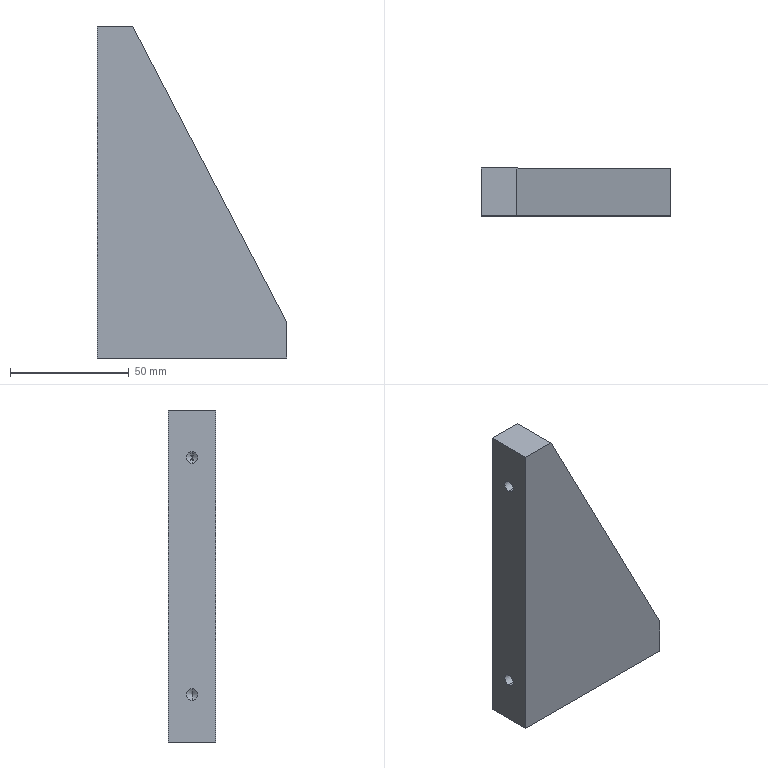Part | SolidWorks | features HoleWzd 2, Extrusion 1, ICE 1 | 1 solid | 23 faces | box 80 x 20 x 140 mm | volume 141533 mm3 | cylinder 8 | cone 8 | plane 7 | commonest cylinder face diameters 5 x8
STEP:
#1=CARTESIAN_POINT('',(75.,10.,-125.));
#2=VERTEX_POINT('',#1);
#3=CARTESIAN_POINT('',(70.,10.,-125.));
#4=VERTEX_POINT('',#3);
#5=CARTESIAN_POINT('',(72.5,10.,-125.));
#6=DIRECTION('',(0.,0.,-1.));
#7=DIRECTION('',(-1.,0.,0.));
#8=AXIS2_PLACEMENT_3D('',#5,#6,#7);
#9=CIRCLE('',#8,2.5);
#10=EDGE_CURVE('',#2,#4,#9,.T.);
#11=ORIENTED_EDGE('',*,*,#10,.F.);
#12=CARTESIAN_POINT('',(75.,10.,-140.));
#13=VERTEX_POINT('',#12);
#14=CARTESIAN_POINT('',(75.,10.,-140.));
#15=DIRECTION('',(0.,0.,-1.));
#16=VECTOR('',#15,1000.);
#17=LINE('',#14,#16);
#18=EDGE_CURVE('',#2,#13,#17,.T.);
#19=ORIENTED_EDGE('',*,*,#18,.T.);
#20=CARTESIAN_POINT('',(70.,10.,-140.));
#21=VERTEX_POINT('',#20);
#22=CARTESIAN_POINT('',(72.5,10.,-140.));
#23=DIRECTION('',(0.,0.,-1.));
#24=DIRECTION('',(-1.,0.,0.));
#25=AXIS2_PLACEMENT_3D('',#22,#23,#24);
#26=CIRCLE('',#25,2.5);
#27=EDGE_CURVE('',#13,#21,#26,.T.);
#28=ORIENTED_EDGE('',*,*,#27,.T.);
#29=CARTESIAN_POINT('',(70.,10.,-140.));
#30=DIRECTION('',(0.,0.,-1.));
#31=VECTOR('',#30,1000.);
#32=LINE('',#29,#31);
#33=EDGE_CURVE('',#4,#21,#32,.T.);
#34=ORIENTED_EDGE('',*,*,#33,.F.);
#35=EDGE_LOOP('',(#11,#19,#28,#34));
#36=FACE_OUTER_BOUND('',#35,.T.);
#37=CARTESIAN_POINT('',(72.5,10.,-140.));
#38=DIRECTION('',(0.,0.,-1.));
#39=DIRECTION('',(-1.,0.,0.));
#40=AXIS2_PLACEMENT_3D('',#37,#38,#39);
#41=CYLINDRICAL_SURFACE('',#40,2.5);
#42=ADVANCED_FACE('',(#36),#41,.F.);
#43=CARTESIAN_POINT('',(72.5,10.,-123.498));
#44=VERTEX_POINT('',#43);
#45=CARTESIAN_POINT('',(70.,10.,-125.));
#46=DIRECTION('',(-0.8572,0.,-0.515));
#47=VECTOR('',#46,1000.);
#48=LINE('',#45,#47);
#49=EDGE_CURVE('',#44,#4,#48,.T.);
#50=ORIENTED_EDGE('',*,*,#49,.F.);
#51=CARTESIAN_POINT('',(75.,10.,-125.));
#52=DIRECTION('',(0.8572,0.,-0.515));
#53=VECTOR('',#52,1000.);
#54=LINE('',#51,#53);
#55=EDGE_CURVE('',#44,#2,#54,.T.);
#56=ORIENTED_EDGE('',*,*,#55,.T.);
#57=ORIENTED_EDGE('',*,*,#10,.T.);
#58=EDGE_LOOP('',(#50,#56,#57));
#59=FACE_OUTER_BOUND('',#58,.T.);
#60=CARTESIAN_POINT('',(72.5,10.,-125.));
#61=DIRECTION('',(0.,0.,-1.));
#62=DIRECTION('',(-1.,0.,0.));
#63=AXIS2_PLACEMENT_3D('',#60,#61,#62);
#64=CONICAL_SURFACE('',#63,2.5,1.03);
#65=ADVANCED_FACE('',(#59),#64,.F.);
#66=CARTESIAN_POINT('',(10.,10.,-125.));
#67=VERTEX_POINT('',#66);
#68=CARTESIAN_POINT('',(5.,10.,-125.));
#69=VERTEX_POINT('',#68);
#70=CARTESIAN_POINT('',(7.5,10.,-125.));
#71=DIRECTION('',(0.,0.,-1.));
#72=DIRECTION('',(-1.,0.,0.));
#73=AXIS2_PLACEMENT_3D('',#70,#71,#72);
#74=CIRCLE('',#73,2.5);
#75=EDGE_CURVE('',#67,#69,#74,.T.);
#76=ORIENTED_EDGE('',*,*,#75,.F.);
#77=CARTESIAN_POINT('',(10.,10.,-140.));
#78=VERTEX_POINT('',#77);
#79=CARTESIAN_POINT('',(10.,10.,-140.));
#80=DIRECTION('',(0.,0.,-1.));
#81=VECTOR('',#80,1000.);
#82=LINE('',#79,#81);
#83=EDGE_CURVE('',#67,#78,#82,.T.);
#84=ORIENTED_EDGE('',*,*,#83,.T.);
#85=CARTESIAN_POINT('',(5.,10.,-140.));
#86=VERTEX_POINT('',#85);
#87=CARTESIAN_POINT('',(7.5,10.,-140.));
#88=DIRECTION('',(0.,0.,-1.));
#89=DIRECTION('',(-1.,0.,0.));
#90=AXIS2_PLACEMENT_3D('',#87,#88,#89);
#91=CIRCLE('',#90,2.5);
#92=EDGE_CURVE('',#78,#86,#91,.T.);
#93=ORIENTED_EDGE('',*,*,#92,.T.);
#94=CARTESIAN_POINT('',(5.,10.,-140.));
#95=DIRECTION('',(0.,0.,-1.));
#96=VECTOR('',#95,1000.);
#97=LINE('',#94,#96);
#98=EDGE_CURVE('',#69,#86,#97,.T.);
#99=ORIENTED_EDGE('',*,*,#98,.F.);
#100=EDGE_LOOP('',(#76,#84,#93,#99));
#101=FACE_OUTER_BOUND('',#100,.T.);
#102=CARTESIAN_POINT('',(7.5,10.,-140.));
#103=DIRECTION('',(0.,0.,-1.));
#104=DIRECTION('',(-1.,0.,0.));
#105=AXIS2_PLACEMENT_3D('',#102,#103,#104);
#106=CYLINDRICAL_SURFACE('',#105,2.5);
#107=ADVANCED_FACE('',(#101),#106,.F.);
#108=CARTESIAN_POINT('',(7.5,10.,-123.498));
#109=VERTEX_POINT('',#108);
#110=CARTESIAN_POINT('',(5.,10.,-125.));
#111=DIRECTION('',(-0.8572,0.,-0.515));
#112=VECTOR('',#111,1000.);
#113=LINE('',#110,#112);
#114=EDGE_CURVE('',#109,#69,#113,.T.);
#115=ORIENTED_EDGE('',*,*,#114,.F.);
#116=CARTESIAN_POINT('',(10.,10.,-125.));
#117=DIRECTION('',(0.8572,0.,-0.515));
#118=VECTOR('',#117,1000.);
#119=LINE('',#116,#118);
#120=EDGE_CURVE('',#109,#67,#119,.T.);
#121=ORIENTED_EDGE('',*,*,#120,.T.);
#122=ORIENTED_EDGE('',*,*,#75,.T.);
#123=EDGE_LOOP('',(#115,#121,#122));
#124=FACE_OUTER_BOUND('',#123,.T.);
#125=CARTESIAN_POINT('',(7.5,10.,-125.));
#126=DIRECTION('',(0.,0.,-1.));
#127=DIRECTION('',(-1.,0.,0.));
#128=AXIS2_PLACEMENT_3D('',#125,#126,#127);
#129=CONICAL_SURFACE('',#128,2.5,1.03);
#130=ADVANCED_FACE('',(#124),#129,.F.);
#131=CARTESIAN_POINT('',(15.,10.,-122.5));
#132=VERTEX_POINT('',#131);
#133=CARTESIAN_POINT('',(15.,10.,-117.5));
#134=VERTEX_POINT('',#133);
#135=CARTESIAN_POINT('',(15.,10.,-120.));
#136=DIRECTION('',(-1.,0.,0.));
#137=DIRECTION('',(0.,0.,1.));
#138=AXIS2_PLACEMENT_3D('',#135,#136,#137);
#139=CIRCLE('',#138,2.5);
#140=EDGE_CURVE('',#132,#134,#139,.T.);
#141=ORIENTED_EDGE('',*,*,#140,.F.);
#142=CARTESIAN_POINT('',(0.,10.,-122.5));
#143=VERTEX_POINT('',#142);
#144=CARTESIAN_POINT('',(0.,10.,-122.5));
#145=DIRECTION('',(-1.,0.,0.));
#146=VECTOR('',#145,1000.);
#147=LINE('',#144,#146);
#148=EDGE_CURVE('',#132,#143,#147,.T.);
#149=ORIENTED_EDGE('',*,*,#148,.T.);
#150=CARTESIAN_POINT('',(0.,10.,-117.5));
#151=VERTEX_POINT('',#150);
#152=CARTESIAN_POINT('',(0.,10.,-120.));
#153=DIRECTION('',(-1.,0.,0.));
#154=DIRECTION('',(0.,0.,1.));
#155=AXIS2_PLACEMENT_3D('',#152,#153,#154);
#156=CIRCLE('',#155,2.5);
#157=EDGE_CURVE('',#143,#151,#156,.T.);
#158=ORIENTED_EDGE('',*,*,#157,.T.);
#159=CARTESIAN_POINT('',(0.,10.,-117.5));
#160=DIRECTION('',(-1.,0.,0.));
#161=VECTOR('',#160,1000.);
#162=LINE('',#159,#161);
#163=EDGE_CURVE('',#134,#151,#162,.T.);
#164=ORIENTED_EDGE('',*,*,#163,.F.);
#165=EDGE_LOOP('',(#141,#149,#158,#164));
#166=FACE_OUTER_BOUND('',#165,.T.);
#167=CARTESIAN_POINT('',(0.,10.,-120.));
#168=DIRECTION('',(-1.,0.,0.));
#169=DIRECTION('',(0.,0.,1.));
#170=AXIS2_PLACEMENT_3D('',#167,#168,#169);
#171=CYLINDRICAL_SURFACE('',#170,2.5);
#172=ADVANCED_FACE('',(#166),#171,.F.);
#173=CARTESIAN_POINT('',(16.502,10.,-120.));
#174=VERTEX_POINT('',#173);
#175=CARTESIAN_POINT('',(15.,10.,-117.5));
#176=DIRECTION('',(-0.515,0.,0.8572));
#177=VECTOR('',#176,1000.);
#178=LINE('',#175,#177);
#179=EDGE_CURVE('',#174,#134,#178,.T.);
#180=ORIENTED_EDGE('',*,*,#179,.F.);
#181=CARTESIAN_POINT('',(15.,10.,-122.5));
#182=DIRECTION('',(-0.515,0.,-0.8572));
#183=VECTOR('',#182,1000.);
#184=LINE('',#181,#183);
#185=EDGE_CURVE('',#174,#132,#184,.T.);
#186=ORIENTED_EDGE('',*,*,#185,.T.);
#187=ORIENTED_EDGE('',*,*,#140,.T.);
#188=EDGE_LOOP('',(#180,#186,#187));
#189=FACE_OUTER_BOUND('',#188,.T.);
#190=CARTESIAN_POINT('',(15.,10.,-120.));
#191=DIRECTION('',(-1.,0.,0.));
#192=DIRECTION('',(0.,0.,1.));
#193=AXIS2_PLACEMENT_3D('',#190,#191,#192);
#194=CONICAL_SURFACE('',#193,2.5,1.03);
#195=ADVANCED_FACE('',(#189),#194,.F.);
#196=CARTESIAN_POINT('',(15.,10.,-22.5));
#197=VERTEX_POINT('',#196);
#198=CARTESIAN_POINT('',(15.,10.,-17.5));
#199=VERTEX_POINT('',#198);
#200=CARTESIAN_POINT('',(15.,10.,-20.));
#201=DIRECTION('',(-1.,0.,0.));
#202=DIRECTION('',(0.,0.,1.));
#203=AXIS2_PLACEMENT_3D('',#200,#201,#202);
#204=CIRCLE('',#203,2.5);
#205=EDGE_CURVE('',#197,#199,#204,.T.);
#206=ORIENTED_EDGE('',*,*,#205,.F.);
#207=CARTESIAN_POINT('',(0.,10.,-22.5));
#208=VERTEX_POINT('',#207);
#209=CARTESIAN_POINT('',(0.,10.,-22.5));
#210=DIRECTION('',(-1.,0.,0.));
#211=VECTOR('',#210,1000.);
#212=LINE('',#209,#211);
#213=EDGE_CURVE('',#197,#208,#212,.T.);
#214=ORIENTED_EDGE('',*,*,#213,.T.);
#215=CARTESIAN_POINT('',(0.,10.,-17.5));
#216=VERTEX_POINT('',#215);
#217=CARTESIAN_POINT('',(0.,10.,-20.));
#218=DIRECTION('',(-1.,0.,0.));
#219=DIRECTION('',(0.,0.,1.));
#220=AXIS2_PLACEMENT_3D('',#217,#218,#219);
#221=CIRCLE('',#220,2.5);
#222=EDGE_CURVE('',#208,#216,#221,.T.);
#223=ORIENTED_EDGE('',*,*,#222,.T.);
#224=CARTESIAN_POINT('',(0.,10.,-17.5));
#225=DIRECTION('',(-1.,0.,0.));
#226=VECTOR('',#225,1000.);
#227=LINE('',#224,#226);
#228=EDGE_CURVE('',#199,#216,#227,.T.);
#229=ORIENTED_EDGE('',*,*,#228,.F.);
#230=EDGE_LOOP('',(#206,#214,#223,#229));
#231=FACE_OUTER_BOUND('',#230,.T.);
#232=CARTESIAN_POINT('',(0.,10.,-20.));
#233=DIRECTION('',(-1.,0.,0.));
#234=DIRECTION('',(0.,0.,1.));
#235=AXIS2_PLACEMENT_3D('',#232,#233,#234);
#236=CYLINDRICAL_SURFACE('',#235,2.5);
#237=ADVANCED_FACE('',(#231),#236,.F.);
#238=CARTESIAN_POINT('',(16.502,10.,-20.));
#239=VERTEX_POINT('',#238);
#240=CARTESIAN_POINT('',(15.,10.,-17.5));
#241=DIRECTION('',(-0.515,0.,0.8572));
#242=VECTOR('',#241,1000.);
#243=LINE('',#240,#242);
#244=EDGE_CURVE('',#239,#199,#243,.T.);
#245=ORIENTED_EDGE('',*,*,#244,.F.);
#246=CARTESIAN_POINT('',(15.,10.,-22.5));
#247=DIRECTION('',(-0.515,0.,-0.8572));
#248=VECTOR('',#247,1000.);
#249=LINE('',#246,#248);
#250=EDGE_CURVE('',#239,#197,#249,.T.);
#251=ORIENTED_EDGE('',*,*,#250,.T.);
#252=ORIENTED_EDGE('',*,*,#205,.T.);
#253=EDGE_LOOP('',(#245,#251,#252));
#254=FACE_OUTER_BOUND('',#253,.T.);
#255=CARTESIAN_POINT('',(15.,10.,-20.));
#256=DIRECTION('',(-1.,0.,0.));
#257=DIRECTION('',(0.,0.,1.));
#258=AXIS2_PLACEMENT_3D('',#255,#256,#257);
#259=CONICAL_SURFACE('',#258,2.5,1.03);
#260=ADVANCED_FACE('',(#254),#259,.F.);
#261=CARTESIAN_POINT('',(15.,0.,0.));
#262=VERTEX_POINT('',#261);
#263=CARTESIAN_POINT('',(15.,20.,0.));
#264=VERTEX_POINT('',#263);
#265=CARTESIAN_POINT('',(15.,0.,0.));
#266=DIRECTION('',(0.,1.,0.));
#267=VECTOR('',#266,1000.);
#268=LINE('',#265,#267);
#269=EDGE_CURVE('',#262,#264,#268,.T.);
#270=ORIENTED_EDGE('',*,*,#269,.T.);
#271=CARTESIAN_POINT('',(0.,20.,0.));
#272=VERTEX_POINT('',#271);
#273=CARTESIAN_POINT('',(0.,20.,0.));
#274=DIRECTION('',(1.,0.,0.));
#275=VECTOR('',#274,1000.);
#276=LINE('',#273,#275);
#277=EDGE_CURVE('',#272,#264,#276,.T.);
#278=ORIENTED_EDGE('',*,*,#277,.F.);
#279=CARTESIAN_POINT('',(0.,0.,0.));
#280=VERTEX_POINT('',#279);
#281=CARTESIAN_POINT('',(0.,20.,0.));
#282=DIRECTION('',(0.,-1.,0.));
#283=VECTOR('',#282,1000.);
#284=LINE('',#281,#283);
#285=EDGE_CURVE('',#272,#280,#284,.T.);
#286=ORIENTED_EDGE('',*,*,#285,.T.);
#287=CARTESIAN_POINT('',(0.,0.,0.));
#288=DIRECTION('',(1.,0.,0.));
#289=VECTOR('',#288,1000.);
#290=LINE('',#287,#289);
#291=EDGE_CURVE('',#280,#262,#290,.T.);
#292=ORIENTED_EDGE('',*,*,#291,.T.);
#293=EDGE_LOOP('',(#270,#278,#286,#292));
#294=FACE_OUTER_BOUND('',#293,.T.);
#295=CARTESIAN_POINT('',(0.,20.,0.));
#296=DIRECTION('',(0.,0.,-1.));
#297=DIRECTION('',(-1.,0.,0.));
#298=AXIS2_PLACEMENT_3D('',#295,#296,#297);
#299=PLANE('',#298);
#300=ADVANCED_FACE('',(#294),#299,.F.);
#301=CARTESIAN_POINT('',(72.5,10.,-140.));
#302=DIRECTION('',(0.,0.,-1.));
#303=DIRECTION('',(-1.,0.,0.));
#304=AXIS2_PLACEMENT_3D('',#301,#302,#303);
#305=CIRCLE('',#304,2.5);
#306=EDGE_CURVE('',#21,#13,#305,.T.);
#307=ORIENTED_EDGE('',*,*,#306,.F.);
#308=ORIENTED_EDGE('',*,*,#27,.F.);
#309=EDGE_LOOP('',(#307,#308));
#310=FACE_BOUND('',#309,.T.);
#311=CARTESIAN_POINT('',(7.5,10.,-140.));
#312=DIRECTION('',(0.,0.,-1.));
#313=DIRECTION('',(-1.,0.,0.));
#314=AXIS2_PLACEMENT_3D('',#311,#312,#313);
#315=CIRCLE('',#314,2.5);
#316=EDGE_CURVE('',#86,#78,#315,.T.);
#317=ORIENTED_EDGE('',*,*,#316,.F.);
#318=ORIENTED_EDGE('',*,*,#92,.F.);
#319=EDGE_LOOP('',(#317,#318));
#320=FACE_BOUND('',#319,.T.);
#321=CARTESIAN_POINT('',(80.,0.,-140.));
#322=VERTEX_POINT('',#321);
#323=CARTESIAN_POINT('',(80.,20.,-140.));
#324=VERTEX_POINT('',#323);
#325=CARTESIAN_POINT('',(80.,0.,-140.));
#326=DIRECTION('',(0.,1.,0.));
#327=VECTOR('',#326,1000.);
#328=LINE('',#325,#327);
#329=EDGE_CURVE('',#322,#324,#328,.T.);
#330=ORIENTED_EDGE('',*,*,#329,.F.);
#331=CARTESIAN_POINT('',(0.,0.,-140.));
#332=VERTEX_POINT('',#331);
#333=CARTESIAN_POINT('',(0.,0.,-140.));
#334=DIRECTION('',(-1.,0.,0.));
#335=VECTOR('',#334,1000.);
#336=LINE('',#333,#335);
#337=EDGE_CURVE('',#322,#332,#336,.T.);
#338=ORIENTED_EDGE('',*,*,#337,.T.);
#339=CARTESIAN_POINT('',(0.,20.,-140.));
#340=VERTEX_POINT('',#339);
#341=CARTESIAN_POINT('',(0.,20.,-140.));
#342=DIRECTION('',(0.,-1.,0.));
#343=VECTOR('',#342,1000.);
#344=LINE('',#341,#343);
#345=EDGE_CURVE('',#340,#332,#344,.T.);
#346=ORIENTED_EDGE('',*,*,#345,.F.);
#347=CARTESIAN_POINT('',(0.,20.,-140.));
#348=DIRECTION('',(-1.,0.,0.));
#349=VECTOR('',#348,1000.);
#350=LINE('',#347,#349);
#351=EDGE_CURVE('',#324,#340,#350,.T.);
#352=ORIENTED_EDGE('',*,*,#351,.F.);
#353=EDGE_LOOP('',(#330,#338,#346,#352));
#354=FACE_OUTER_BOUND('',#353,.T.);
#355=CARTESIAN_POINT('',(0.,20.,-140.));
#356=DIRECTION('',(0.,0.,1.));
#357=DIRECTION('',(1.,0.,0.));
#358=AXIS2_PLACEMENT_3D('',#355,#356,#357);
#359=PLANE('',#358);
#360=ADVANCED_FACE('',(#310,#320,#354),#359,.F.);
#361=CARTESIAN_POINT('',(80.,20.,-125.));
#362=VERTEX_POINT('',#361);
#363=CARTESIAN_POINT('',(80.,20.,-140.));
#364=DIRECTION('',(0.,0.,-1.));
#365=VECTOR('',#364,1000.);
#366=LINE('',#363,#365);
#367=EDGE_CURVE('',#362,#324,#366,.T.);
#368=ORIENTED_EDGE('',*,*,#367,.T.);
#369=ORIENTED_EDGE('',*,*,#351,.T.);
#370=CARTESIAN_POINT('',(0.,20.,0.));
#371=DIRECTION('',(0.,0.,1.));
#372=VECTOR('',#371,1000.);
#373=LINE('',#370,#372);
#374=EDGE_CURVE('',#340,#272,#373,.T.);
#375=ORIENTED_EDGE('',*,*,#374,.T.);
#376=ORIENTED_EDGE('',*,*,#277,.T.);
#377=CARTESIAN_POINT('',(80.,20.,-125.));
#378=DIRECTION('',(0.4614,0.,-0.8872));
#379=VECTOR('',#378,1000.);
#380=LINE('',#377,#379);
#381=EDGE_CURVE('',#264,#362,#380,.T.);
#382=ORIENTED_EDGE('',*,*,#381,.T.);
#383=EDGE_LOOP('',(#368,#369,#375,#376,#382));
#384=FACE_OUTER_BOUND('',#383,.T.);
#385=CARTESIAN_POINT('',(0.,20.,0.));
#386=DIRECTION('',(0.,-1.,0.));
#387=DIRECTION('',(0.,0.,-1.));
#388=AXIS2_PLACEMENT_3D('',#385,#386,#387);
#389=PLANE('',#388);
#390=ADVANCED_FACE('',(#384),#389,.F.);
#391=ORIENTED_EDGE('',*,*,#337,.F.);
#392=CARTESIAN_POINT('',(80.,0.,-125.));
#393=VERTEX_POINT('',#392);
#394=CARTESIAN_POINT('',(80.,0.,-140.));
#395=DIRECTION('',(0.,0.,-1.));
#396=VECTOR('',#395,1000.);
#397=LINE('',#394,#396);
#398=EDGE_CURVE('',#393,#322,#397,.T.);
#399=ORIENTED_EDGE('',*,*,#398,.F.);
#400=CARTESIAN_POINT('',(80.,0.,-125.));
#401=DIRECTION('',(0.4614,0.,-0.8872));
#402=VECTOR('',#401,1000.);
#403=LINE('',#400,#402);
#404=EDGE_CURVE('',#262,#393,#403,.T.);
#405=ORIENTED_EDGE('',*,*,#404,.F.);
#406=ORIENTED_EDGE('',*,*,#291,.F.);
#407=CARTESIAN_POINT('',(0.,0.,0.));
#408=DIRECTION('',(0.,0.,1.));
#409=VECTOR('',#408,1000.);
#410=LINE('',#407,#409);
#411=EDGE_CURVE('',#332,#280,#410,.T.);
#412=ORIENTED_EDGE('',*,*,#411,.F.);
#413=EDGE_LOOP('',(#391,#399,#405,#406,#412));
#414=FACE_OUTER_BOUND('',#413,.T.);
#415=CARTESIAN_POINT('',(0.,0.,0.));
#416=DIRECTION('',(0.,-1.,0.));
#417=DIRECTION('',(0.,0.,-1.));
#418=AXIS2_PLACEMENT_3D('',#415,#416,#417);
#419=PLANE('',#418);
#420=ADVANCED_FACE('',(#414),#419,.T.);
#421=CARTESIAN_POINT('',(0.,10.,-120.));
#422=DIRECTION('',(-1.,0.,0.));
#423=DIRECTION('',(0.,0.,1.));
#424=AXIS2_PLACEMENT_3D('',#421,#422,#423);
#425=CIRCLE('',#424,2.5);
#426=EDGE_CURVE('',#151,#143,#425,.T.);
#427=ORIENTED_EDGE('',*,*,#426,.F.);
#428=ORIENTED_EDGE('',*,*,#157,.F.);
#429=EDGE_LOOP('',(#427,#428));
#430=FACE_BOUND('',#429,.T.);
#431=CARTESIAN_POINT('',(0.,10.,-20.));
#432=DIRECTION('',(-1.,0.,0.));
#433=DIRECTION('',(0.,0.,1.));
#434=AXIS2_PLACEMENT_3D('',#431,#432,#433);
#435=CIRCLE('',#434,2.5);
#436=EDGE_CURVE('',#216,#208,#435,.T.);
#437=ORIENTED_EDGE('',*,*,#436,.F.);
#438=ORIENTED_EDGE('',*,*,#222,.F.);
#439=EDGE_LOOP('',(#437,#438));
#440=FACE_BOUND('',#439,.T.);
#441=ORIENTED_EDGE('',*,*,#411,.T.);
#442=ORIENTED_EDGE('',*,*,#285,.F.);
#443=ORIENTED_EDGE('',*,*,#374,.F.);
#444=ORIENTED_EDGE('',*,*,#345,.T.);
#445=EDGE_LOOP('',(#441,#442,#443,#444));
#446=FACE_OUTER_BOUND('',#445,.T.);
#447=CARTESIAN_POINT('',(0.,20.,0.));
#448=DIRECTION('',(1.,0.,0.));
#449=DIRECTION('',(0.,0.,-1.));
#450=AXIS2_PLACEMENT_3D('',#447,#448,#449);
#451=PLANE('',#450);
#452=ADVANCED_FACE('',(#430,#440,#446),#451,.F.);
#453=ORIENTED_EDGE('',*,*,#367,.F.);
#454=CARTESIAN_POINT('',(80.,0.,-125.));
#455=DIRECTION('',(0.,1.,0.));
#456=VECTOR('',#455,1000.);
#457=LINE('',#454,#456);
#458=EDGE_CURVE('',#393,#362,#457,.T.);
#459=ORIENTED_EDGE('',*,*,#458,.F.);
#460=ORIENTED_EDGE('',*,*,#398,.T.);
#461=ORIENTED_EDGE('',*,*,#329,.T.);
#462=EDGE_LOOP('',(#453,#459,#460,#461));
#463=FACE_OUTER_BOUND('',#462,.T.);
#464=CARTESIAN_POINT('',(80.,0.,-140.));
#465=DIRECTION('',(1.,0.,0.));
#466=DIRECTION('',(0.,0.,-1.));
#467=AXIS2_PLACEMENT_3D('',#464,#465,#466);
#468=PLANE('',#467);
#469=ADVANCED_FACE('',(#463),#468,.T.);
#470=ORIENTED_EDGE('',*,*,#381,.F.);
#471=ORIENTED_EDGE('',*,*,#269,.F.);
#472=ORIENTED_EDGE('',*,*,#404,.T.);
#473=ORIENTED_EDGE('',*,*,#458,.T.);
#474=EDGE_LOOP('',(#470,#471,#472,#473));
#475=FACE_OUTER_BOUND('',#474,.T.);
#476=CARTESIAN_POINT('',(80.,0.,-125.));
#477=DIRECTION('',(0.8872,0.,0.4614));
#478=DIRECTION('',(0.4614,0.,-0.8872));
#479=AXIS2_PLACEMENT_3D('',#476,#477,#478);
#480=PLANE('',#479);
#481=ADVANCED_FACE('',(#475),#480,.T.);
#482=ORIENTED_EDGE('',*,*,#250,.F.);
#483=ORIENTED_EDGE('',*,*,#244,.T.);
#484=CARTESIAN_POINT('',(15.,10.,-20.));
#485=DIRECTION('',(-1.,0.,0.));
#486=DIRECTION('',(0.,0.,1.));
#487=AXIS2_PLACEMENT_3D('',#484,#485,#486);
#488=CIRCLE('',#487,2.5);
#489=EDGE_CURVE('',#199,#197,#488,.T.);
#490=ORIENTED_EDGE('',*,*,#489,.T.);
#491=EDGE_LOOP('',(#482,#483,#490));
#492=FACE_OUTER_BOUND('',#491,.T.);
#493=CARTESIAN_POINT('',(15.,10.,-20.));
#494=DIRECTION('',(-1.,0.,0.));
#495=DIRECTION('',(0.,0.,1.));
#496=AXIS2_PLACEMENT_3D('',#493,#494,#495);
#497=CONICAL_SURFACE('',#496,2.5,1.03);
#498=ADVANCED_FACE('',(#492),#497,.F.);
#499=ORIENTED_EDGE('',*,*,#213,.F.);
#500=ORIENTED_EDGE('',*,*,#489,.F.);
#501=ORIENTED_EDGE('',*,*,#228,.T.);
#502=ORIENTED_EDGE('',*,*,#436,.T.);
#503=EDGE_LOOP('',(#499,#500,#501,#502));
#504=FACE_OUTER_BOUND('',#503,.T.);
#505=CARTESIAN_POINT('',(0.,10.,-20.));
#506=DIRECTION('',(-1.,0.,0.));
#507=DIRECTION('',(0.,0.,1.));
#508=AXIS2_PLACEMENT_3D('',#505,#506,#507);
#509=CYLINDRICAL_SURFACE('',#508,2.5);
#510=ADVANCED_FACE('',(#504),#509,.F.);
#511=ORIENTED_EDGE('',*,*,#185,.F.);
#512=ORIENTED_EDGE('',*,*,#179,.T.);
#513=CARTESIAN_POINT('',(15.,10.,-120.));
#514=DIRECTION('',(-1.,0.,0.));
#515=DIRECTION('',(0.,0.,1.));
#516=AXIS2_PLACEMENT_3D('',#513,#514,#515);
#517=CIRCLE('',#516,2.5);
#518=EDGE_CURVE('',#134,#132,#517,.T.);
#519=ORIENTED_EDGE('',*,*,#518,.T.);
#520=EDGE_LOOP('',(#511,#512,#519));
#521=FACE_OUTER_BOUND('',#520,.T.);
#522=CARTESIAN_POINT('',(15.,10.,-120.));
#523=DIRECTION('',(-1.,0.,0.));
#524=DIRECTION('',(0.,0.,1.));
#525=AXIS2_PLACEMENT_3D('',#522,#523,#524);
#526=CONICAL_SURFACE('',#525,2.5,1.03);
#527=ADVANCED_FACE('',(#521),#526,.F.);
#528=ORIENTED_EDGE('',*,*,#148,.F.);
#529=ORIENTED_EDGE('',*,*,#518,.F.);
#530=ORIENTED_EDGE('',*,*,#163,.T.);
#531=ORIENTED_EDGE('',*,*,#426,.T.);
#532=EDGE_LOOP('',(#528,#529,#530,#531));
#533=FACE_OUTER_BOUND('',#532,.T.);
#534=CARTESIAN_POINT('',(0.,10.,-120.));
#535=DIRECTION('',(-1.,0.,0.));
#536=DIRECTION('',(0.,0.,1.));
#537=AXIS2_PLACEMENT_3D('',#534,#535,#536);
#538=CYLINDRICAL_SURFACE('',#537,2.5);
#539=ADVANCED_FACE('',(#533),#538,.F.);
#540=ORIENTED_EDGE('',*,*,#120,.F.);
#541=ORIENTED_EDGE('',*,*,#114,.T.);
#542=CARTESIAN_POINT('',(7.5,10.,-125.));
#543=DIRECTION('',(0.,0.,-1.));
#544=DIRECTION('',(-1.,0.,0.));
#545=AXIS2_PLACEMENT_3D('',#542,#543,#544);
#546=CIRCLE('',#545,2.5);
#547=EDGE_CURVE('',#69,#67,#546,.T.);
#548=ORIENTED_EDGE('',*,*,#547,.T.);
#549=EDGE_LOOP('',(#540,#541,#548));
#550=FACE_OUTER_BOUND('',#549,.T.);
#551=CARTESIAN_POINT('',(7.5,10.,-125.));
#552=DIRECTION('',(0.,0.,-1.));
#553=DIRECTION('',(-1.,0.,0.));
#554=AXIS2_PLACEMENT_3D('',#551,#552,#553);
#555=CONICAL_SURFACE('',#554,2.5,1.03);
#556=ADVANCED_FACE('',(#550),#555,.F.);
#557=ORIENTED_EDGE('',*,*,#83,.F.);
#558=ORIENTED_EDGE('',*,*,#547,.F.);
#559=ORIENTED_EDGE('',*,*,#98,.T.);
#560=ORIENTED_EDGE('',*,*,#316,.T.);
#561=EDGE_LOOP('',(#557,#558,#559,#560));
#562=FACE_OUTER_BOUND('',#561,.T.);
#563=CARTESIAN_POINT('',(7.5,10.,-140.));
#564=DIRECTION('',(0.,0.,-1.));
#565=DIRECTION('',(-1.,0.,0.));
#566=AXIS2_PLACEMENT_3D('',#563,#564,#565);
#567=CYLINDRICAL_SURFACE('',#566,2.5);
#568=ADVANCED_FACE('',(#562),#567,.F.);
#569=ORIENTED_EDGE('',*,*,#55,.F.);
#570=ORIENTED_EDGE('',*,*,#49,.T.);
#571=CARTESIAN_POINT('',(72.5,10.,-125.));
#572=DIRECTION('',(0.,0.,-1.));
#573=DIRECTION('',(-1.,0.,0.));
#574=AXIS2_PLACEMENT_3D('',#571,#572,#573);
#575=CIRCLE('',#574,2.5);
#576=EDGE_CURVE('',#4,#2,#575,.T.);
#577=ORIENTED_EDGE('',*,*,#576,.T.);
#578=EDGE_LOOP('',(#569,#570,#577));
#579=FACE_OUTER_BOUND('',#578,.T.);
#580=CARTESIAN_POINT('',(72.5,10.,-125.));
#581=DIRECTION('',(0.,0.,-1.));
#582=DIRECTION('',(-1.,0.,0.));
#583=AXIS2_PLACEMENT_3D('',#580,#581,#582);
#584=CONICAL_SURFACE('',#583,2.5,1.03);
#585=ADVANCED_FACE('',(#579),#584,.F.);
#586=ORIENTED_EDGE('',*,*,#18,.F.);
#587=ORIENTED_EDGE('',*,*,#576,.F.);
#588=ORIENTED_EDGE('',*,*,#33,.T.);
#589=ORIENTED_EDGE('',*,*,#306,.T.);
#590=EDGE_LOOP('',(#586,#587,#588,#589));
#591=FACE_OUTER_BOUND('',#590,.T.);
#592=CARTESIAN_POINT('',(72.5,10.,-140.));
#593=DIRECTION('',(0.,0.,-1.));
#594=DIRECTION('',(-1.,0.,0.));
#595=AXIS2_PLACEMENT_3D('',#592,#593,#594);
#596=CYLINDRICAL_SURFACE('',#595,2.5);
#597=ADVANCED_FACE('',(#591),#596,.F.);
#598=CLOSED_SHELL('',(#42,#65,#107,#130,#172,#195,#237,#260,#300,#360,#390,#420,#452,#469,#481,#498,#510,#527,#539,#556,#568,#585,#597));
#599=MANIFOLD_SOLID_BREP('',#598);
#600=CARTESIAN_POINT('',(0.,0.,0.));
#601=DIRECTION('',(0.,0.,1.));
#602=DIRECTION('',(1.,0.,0.));
#603=AXIS2_PLACEMENT_3D('',#600,#601,#602);
#604=(LENGTH_UNIT()NAMED_UNIT(*)SI_UNIT(.MILLI.,.METRE.));
#605=UNCERTAINTY_MEASURE_WITH_UNIT(LENGTH_MEASURE(0.00001),#604,'','');
#606=(NAMED_UNIT(*)PLANE_ANGLE_UNIT()SI_UNIT($,.RADIAN.));
#607=(NAMED_UNIT(*)SI_UNIT($,.STERADIAN.)SOLID_ANGLE_UNIT());
#608=(GEOMETRIC_REPRESENTATION_CONTEXT(3)GLOBAL_UNCERTAINTY_ASSIGNED_CONTEXT((#605))GLOBAL_UNIT_ASSIGNED_CONTEXT((#604,#606,#607))REPRESENTATION_CONTEXT('',''));
#609=ADVANCED_BREP_SHAPE_REPRESENTATION('',(#599,#603),#608);